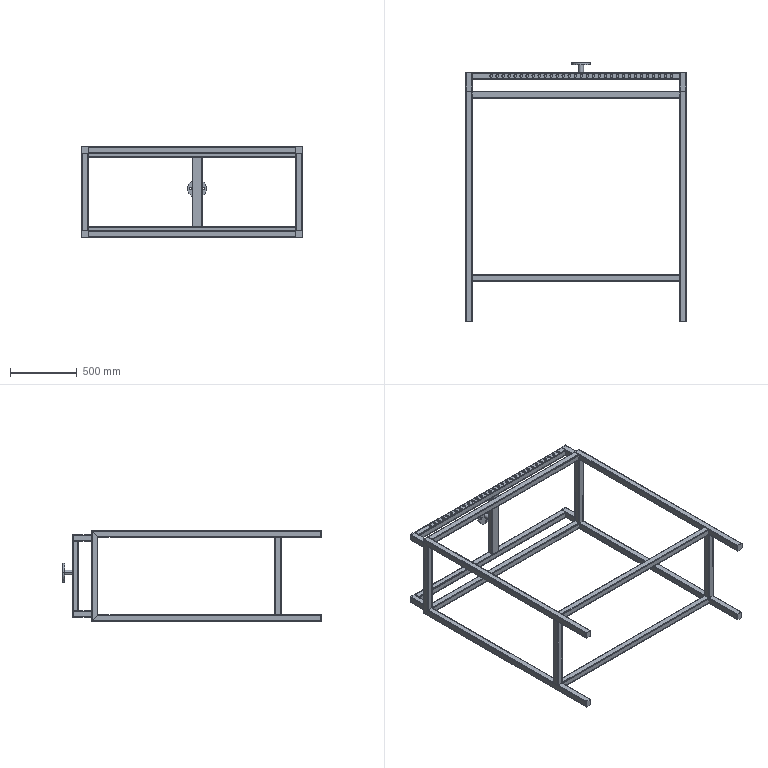Part | SolidWorks | features AEMSimFeature 1 | 20 solids | 494 faces | box 1650 x 1942 x 680 mm | volume 17460157 mm3 | cylinder 292 | plane 202 | commonest cylinder face diameters 20 x124 2 x76 12 x76 18 x8 38 x2 39 x2